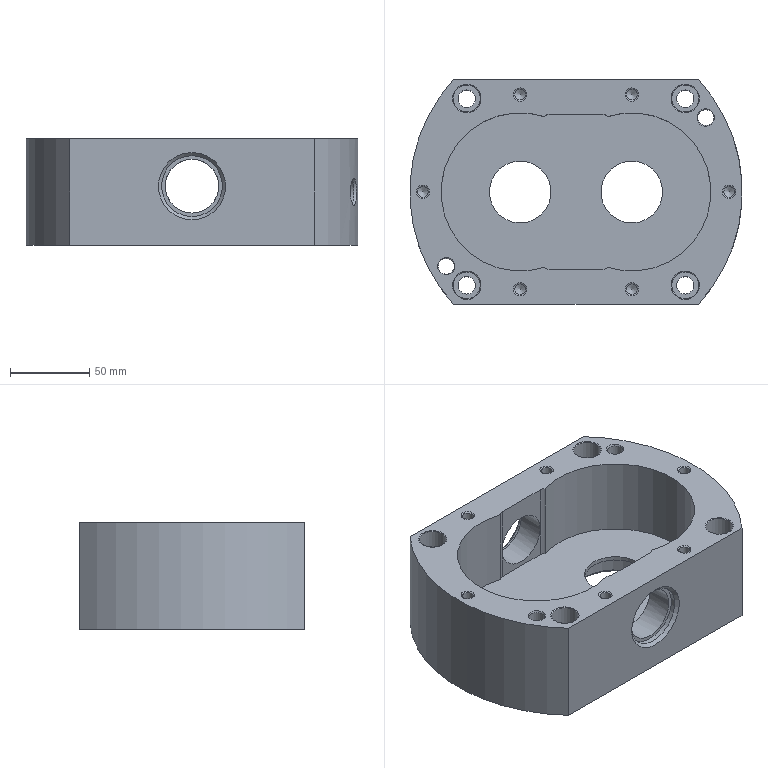NC program | NX | posted with a generic post | part box 210 x 142 x 67.4 mm
Lines 1 to 85 of 83330:
N10 G17 G21 G94 G90
(DRILLING , TOOL : ZXZ)
N12 T01 M6
N14 G54
N16 G17 G0 G90 X69. Y59. B0. C0. S5000 M3
N18 G43 Z30. H1
N20 G94 G81 G98 Z-1. F250. R3.
N22 X60.706 Y25.456
N24 X35.25 Y0.
N26 X60.706 Y-25.456
N28 X82. Y-47.
N30 X69. Y-59.
N32 X9.794 Y-25.456
N34 X-9.794
N36 X9.794 Y25.456
N38 X-9.794
N40 X-69. Y59.
N42 X-82. Y47.
N44 X-60.706 Y25.456
N46 X-35.25 Y0.
N48 X-60.706 Y-25.456
N50 X-69. Y-59.
N52 G80
N54 G0 X-69. Y-59. Z30.
N56 M5
(DRILLING_COPY , TOOL : 11.0ZT)
N58 T09 M6
N60 G54
N62 G17 G0 G90 X-69. Y59. B0. C0. S2000 M3
N64 G43 Z30. H9
N66 G94 G83 G98 Z-70.705 F150. Q2. R3.
N68 Y-59.
N70 X69.
N72 Y59.
N74 G80
N76 G0 X69. Y59. Z30.
N78 M5
(DRILLING_COPY_COPY , TOOL : 9.8ZT)
N80 T19 M6
N82 G54
N84 G17 G0 G90 X-82. Y47. B0. C0. S2000 M3
N86 G43 Z30. H19
N88 G94 G83 G98 Z-71.844 F150. Q2. R3.
N90 X82. Y-47.
N92 G80
N94 G0 X82. Y-47. Z30.
N96 M5
(DRILLING_COPY_COPY_COPY , TOOL : 10.0JD)
N98 T17 M6
N100 G54
N102 G17 G0 G90 X-82. Y47. B0. C0. S800 M3
N104 G43 Z30. H17
N106 G94 G85 G98 Z-67.9 F40. R3.
N108 X82. Y-47.
N110 G80
N112 G0 X82. Y-47. Z30.
N114 M5
(DRILLING_COPY_COPY_1 , TOOL : 4.2ZT)
N116 T15 M6
N118 G54
N120 G17 G0 G90 X60.706 Y25.456 B0. C0. S2000 M3
N122 G43 Z30. H15
N124 G94 G83 G98 Z-14.262 F150. Q2. R3.
N126 Y-25.456
N128 X9.794
N130 X-9.794
N132 X-60.706
N134 Y25.456
N136 X-9.794
N138 X9.794
N140 G80
N142 G0 X9.794 Y25.456 Z30.
N144 M5